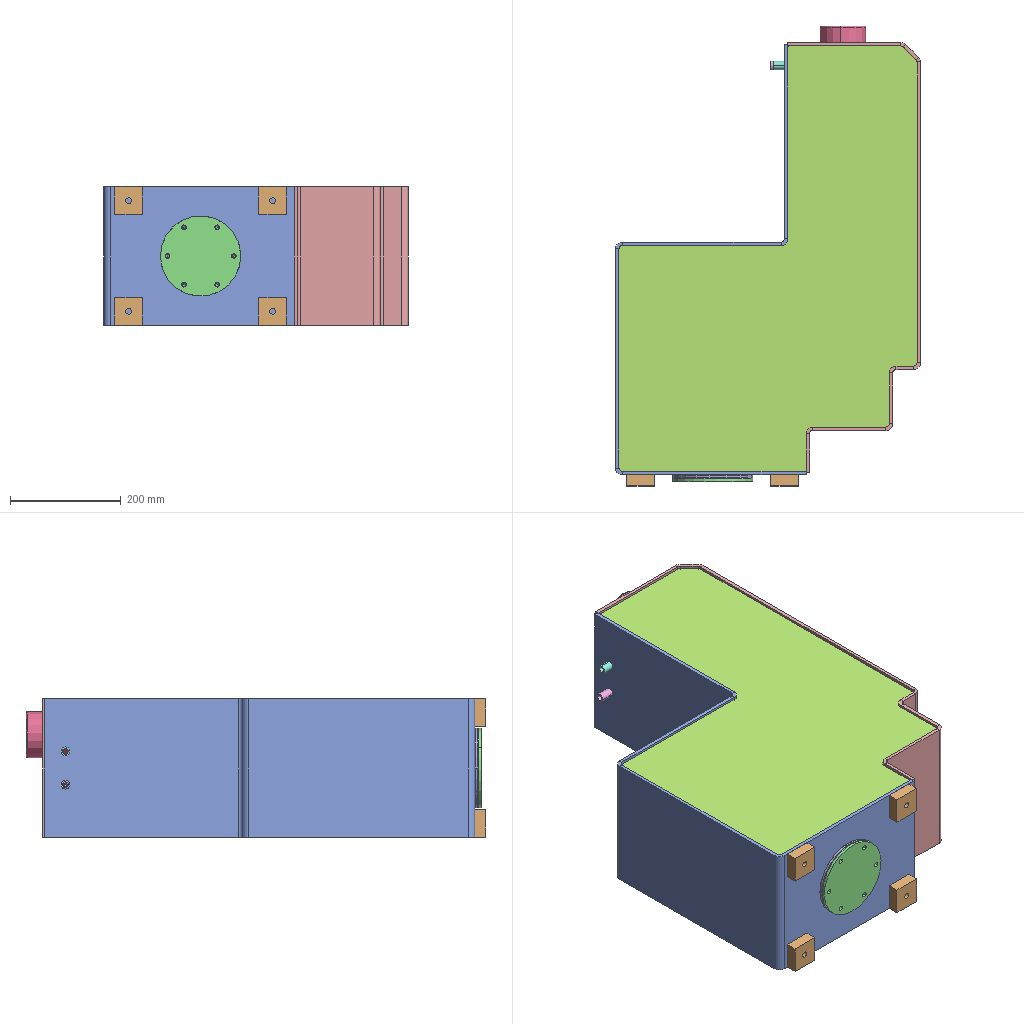Assembly | SolidWorks | 10 different items | 14 placed | box 550 x 830 x 250 mm
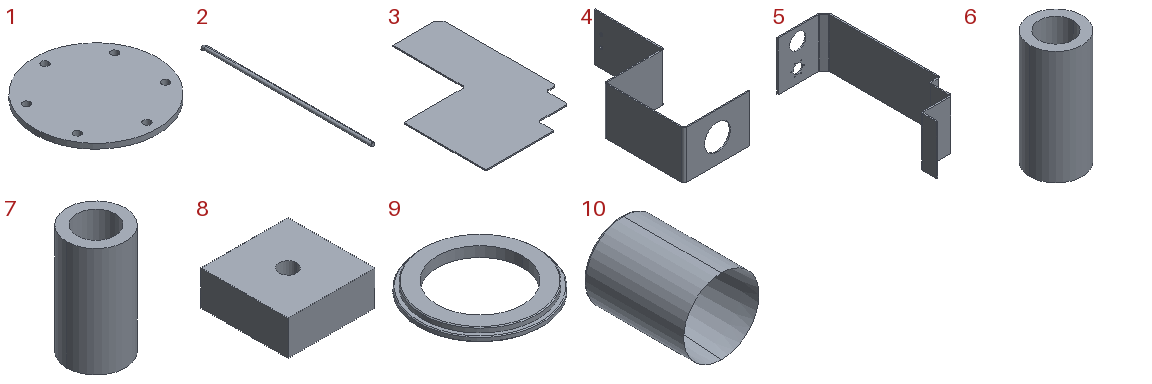Parts list (item | quantity | size | volume | features):
1 | x1 | 145 x 145 x 6 mm | 97035 mm3 | features Extrusion 1
2 | x1 | 16 x 738 x 18 mm | 127006 mm3 | features ICE 2, Sweep 1
3 | x2 | 538 x 768 x 6 mm | 1689315 mm3 | features FlatPattern 1, SMBaseFlange 1, SheetMetal 1
4 | x1 | 344 x 776 x 250 mm | 2022821 mm3 | features ICE 2, FlatPattern 1, SMBaseFlange 1, SheetMetal 1
5 | x1 | 239 x 776 x 250 mm | 1720525 mm3 | features FlatPattern 1, HoleWzd 1, ICE 1, SMBaseFlange 1, SheetMetal 1
6 | x1 | 16 x 16 x 35 mm | 4007 mm3 | features Extrusion 1, HoleWzd 1
7 | x1 | 16 x 16 x 30 mm | 3434 mm3 | features Extrusion 1, HoleWzd 1
8 | x4 | 50 x 50 x 20 mm | 48366 mm3 | features FlatPattern 1, HoleWzd 1, SMBaseFlange 1, SheetMetal 1
9 | x1 | 145 x 145 x 12 mm | 88157 mm3 | features ICE 2, Chamfer 1, Extrusion 1, HoleWzd 1
10 | x1 | 83 x 110 x 83 mm | 48850 mm3 | features RevolutionThin 1
Mates (type | each side: item.copy, entity, surface, feature):
Coincident | 5.1 face plane Base-Flange1 | 4.1 face plane Base-Flange1 | 2 times
DistanceDim | 5.1 face plane Base-Flange1 | 4.1 face plane Base-Flange1
InPlace | 3.1 plane | assembly plane
Concentric | 4.1 face cylinder Cut-Extrude1 | 6.1 face cylinder Boss-Extrude1
DistanceDim | 6.1 face plane Boss-Extrude1 | 4.1 face plane Base-Flange1
Concentric | 4.1 face cylinder Cut-Extrude1 | 7.1 face cylinder Boss-Extrude1
DistanceDim | 4.1 face plane Base-Flange1 | 7.1 face plane Boss-Extrude1
Parallel | 6.1 plane | assembly plane
Parallel | 7.1 plane | assembly plane
Coincident | 4.1 face plane Base-Flange1 | 8.1 face plane Base-Flange1 | 2 times
DistanceDim | 8.1 face plane Base-Flange1 | 4.1 face plane Base-Flange1
Coincident | 4.1 face plane Base-Flange1 | 9.1 face plane Boss-Extrude1
Concentric | 4.1 face cylinder Cut-Extrude2 | 9.1 face cylinder Boss-Extrude1
Parallel | 9.1 plane | assembly plane
Coincident | 9.1 face plane Boss-Extrude1 | 1.1 face plane Boss-Extrude1
Concentric | 9.1 face cylinder Boss-Extrude1 | 1.1 face cylinder Boss-Extrude1
Concentric | 9.1 face cylinder M8 Tapped Hole1 | 1.1 face cylinder Boss-Extrude1
Concentric | 5.1 face cylinder Cut-Extrude1 | 10.1 face cylinder Revolve-Thin1
DistanceDim | 10.1 face plane Revolve-Thin1 | 5.1 face plane Base-Flange1
Coincident | 6.1 face plane Boss-Extrude1 | 2.1 face plane Sweep1
Concentric | 6.1 edge | 2.1 edge